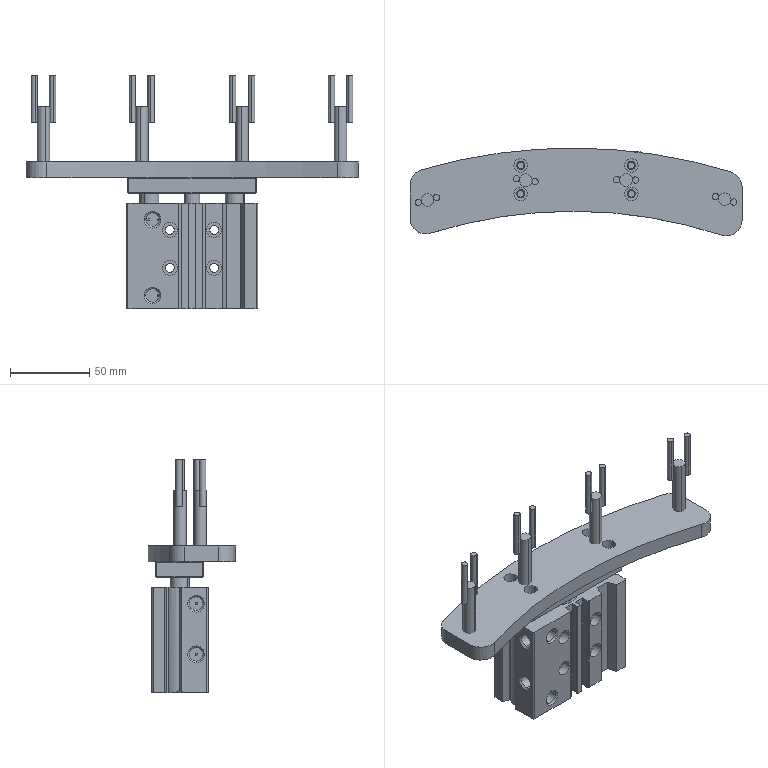Part | 26 solids | 634 faces | box 210 x 55.542 x 148 mm | volume 271199 mm3 | cylinder 287 | plane 229 | cone 103 | torus 12 | spline 3 | commonest cylinder face diameters 5 x45 8 x20 4.2 x18 1.5 x16 4 x16 3 x12